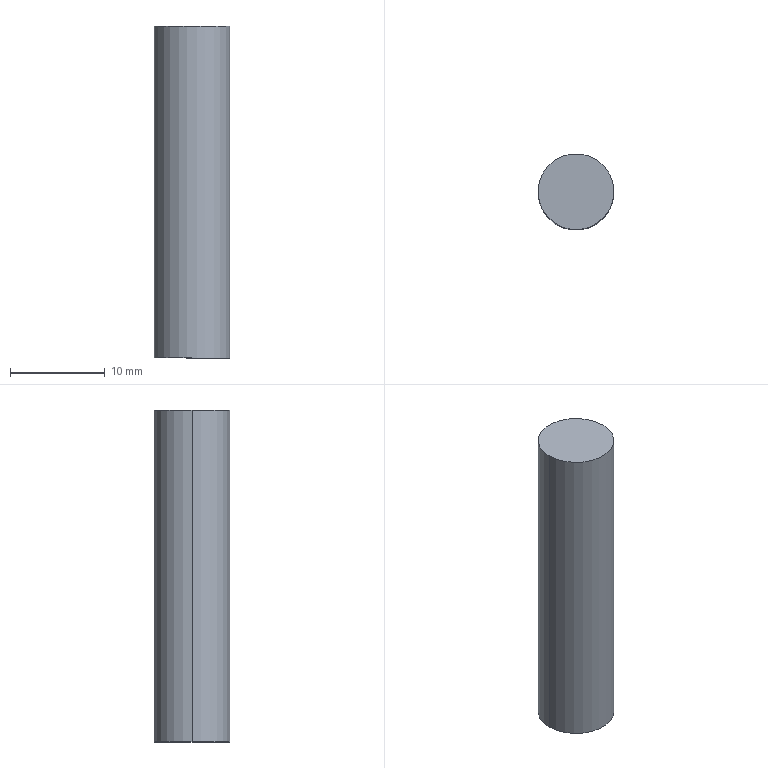Part | SolidWorks | features BaseBody 1 | 1 solid | 4 faces | box 8 x 8 x 35 mm | volume 1759 mm3 | cylinder 2 | plane 2 | commonest cylinder face diameters 8 x2
STEP:
#1=CARTESIAN_POINT('',(-863.,42.5,35.5));
#2=VERTEX_POINT('',#1);
#3=CARTESIAN_POINT('',(-855.,42.5,35.5));
#4=VERTEX_POINT('',#3);
#5=CARTESIAN_POINT('',(-859.,42.5,35.5));
#6=DIRECTION('',(0.,0.,-1.));
#7=DIRECTION('',(-1.,0.,0.));
#8=AXIS2_PLACEMENT_3D('',#5,#6,#7);
#9=CIRCLE('',#8,4.);
#10=EDGE_CURVE('',#2,#4,#9,.T.);
#11=ORIENTED_EDGE('',*,*,#10,.T.);
#12=CARTESIAN_POINT('',(-855.,42.5,0.5));
#13=VERTEX_POINT('',#12);
#14=CARTESIAN_POINT('',(-855.,42.5,0.5));
#15=DIRECTION('',(0.,0.,-1.));
#16=VECTOR('',#15,1000.);
#17=LINE('',#14,#16);
#18=EDGE_CURVE('',#4,#13,#17,.T.);
#19=ORIENTED_EDGE('',*,*,#18,.T.);
#20=CARTESIAN_POINT('',(-863.,42.5,0.5));
#21=VERTEX_POINT('',#20);
#22=CARTESIAN_POINT('',(-859.,42.5,0.5));
#23=DIRECTION('',(0.,0.,1.));
#24=DIRECTION('',(-1.,0.,0.));
#25=AXIS2_PLACEMENT_3D('',#22,#23,#24);
#26=CIRCLE('',#25,4.);
#27=EDGE_CURVE('',#13,#21,#26,.T.);
#28=ORIENTED_EDGE('',*,*,#27,.T.);
#29=CARTESIAN_POINT('',(-863.,42.5,0.5));
#30=DIRECTION('',(0.,0.,-1.));
#31=VECTOR('',#30,1000.);
#32=LINE('',#29,#31);
#33=EDGE_CURVE('',#2,#21,#32,.T.);
#34=ORIENTED_EDGE('',*,*,#33,.F.);
#35=EDGE_LOOP('',(#11,#19,#28,#34));
#36=FACE_OUTER_BOUND('',#35,.T.);
#37=CARTESIAN_POINT('',(-859.,42.5,0.5));
#38=DIRECTION('',(0.,0.,-1.));
#39=DIRECTION('',(-1.,0.,0.));
#40=AXIS2_PLACEMENT_3D('',#37,#38,#39);
#41=CYLINDRICAL_SURFACE('',#40,4.);
#42=ADVANCED_FACE('',(#36),#41,.T.);
#43=ORIENTED_EDGE('',*,*,#18,.F.);
#44=CARTESIAN_POINT('',(-859.,42.5,35.5));
#45=DIRECTION('',(0.,0.,-1.));
#46=DIRECTION('',(-1.,0.,0.));
#47=AXIS2_PLACEMENT_3D('',#44,#45,#46);
#48=CIRCLE('',#47,4.);
#49=EDGE_CURVE('',#4,#2,#48,.T.);
#50=ORIENTED_EDGE('',*,*,#49,.T.);
#51=ORIENTED_EDGE('',*,*,#33,.T.);
#52=CARTESIAN_POINT('',(-859.,42.5,0.5));
#53=DIRECTION('',(0.,0.,1.));
#54=DIRECTION('',(-1.,0.,0.));
#55=AXIS2_PLACEMENT_3D('',#52,#53,#54);
#56=CIRCLE('',#55,4.);
#57=EDGE_CURVE('',#21,#13,#56,.T.);
#58=ORIENTED_EDGE('',*,*,#57,.T.);
#59=EDGE_LOOP('',(#43,#50,#51,#58));
#60=FACE_OUTER_BOUND('',#59,.T.);
#61=CARTESIAN_POINT('',(-859.,42.5,0.5));
#62=DIRECTION('',(0.,0.,-1.));
#63=DIRECTION('',(-1.,0.,0.));
#64=AXIS2_PLACEMENT_3D('',#61,#62,#63);
#65=CYLINDRICAL_SURFACE('',#64,4.);
#66=ADVANCED_FACE('',(#60),#65,.T.);
#67=ORIENTED_EDGE('',*,*,#57,.F.);
#68=ORIENTED_EDGE('',*,*,#27,.F.);
#69=EDGE_LOOP('',(#67,#68));
#70=FACE_OUTER_BOUND('',#69,.T.);
#71=CARTESIAN_POINT('',(-860.608,42.5,0.5));
#72=DIRECTION('',(0.,0.,-1.));
#73=DIRECTION('',(0.,1.,0.));
#74=AXIS2_PLACEMENT_3D('',#71,#72,#73);
#75=PLANE('',#74);
#76=ADVANCED_FACE('',(#70),#75,.T.);
#77=ORIENTED_EDGE('',*,*,#10,.F.);
#78=ORIENTED_EDGE('',*,*,#49,.F.);
#79=EDGE_LOOP('',(#77,#78));
#80=FACE_OUTER_BOUND('',#79,.T.);
#81=CARTESIAN_POINT('',(-860.608,42.5,35.5));
#82=DIRECTION('',(0.,0.,1.));
#83=DIRECTION('',(1.,0.,0.));
#84=AXIS2_PLACEMENT_3D('',#81,#82,#83);
#85=PLANE('',#84);
#86=ADVANCED_FACE('',(#80),#85,.T.);
#87=CLOSED_SHELL('',(#42,#66,#76,#86));
#88=MANIFOLD_SOLID_BREP('',#87);
#89=CARTESIAN_POINT('',(0.,0.,0.));
#90=DIRECTION('',(0.,0.,1.));
#91=DIRECTION('',(1.,0.,0.));
#92=AXIS2_PLACEMENT_3D('',#89,#90,#91);
#93=(LENGTH_UNIT()NAMED_UNIT(*)SI_UNIT(.MILLI.,.METRE.));
#94=UNCERTAINTY_MEASURE_WITH_UNIT(LENGTH_MEASURE(0.00001),#93,'','');
#95=(NAMED_UNIT(*)PLANE_ANGLE_UNIT()SI_UNIT($,.RADIAN.));
#96=(NAMED_UNIT(*)SI_UNIT($,.STERADIAN.)SOLID_ANGLE_UNIT());
#97=(GEOMETRIC_REPRESENTATION_CONTEXT(3)GLOBAL_UNCERTAINTY_ASSIGNED_CONTEXT((#94))GLOBAL_UNIT_ASSIGNED_CONTEXT((#93,#95,#96))REPRESENTATION_CONTEXT('',''));
#98=ADVANCED_BREP_SHAPE_REPRESENTATION('',(#88,#92),#97);